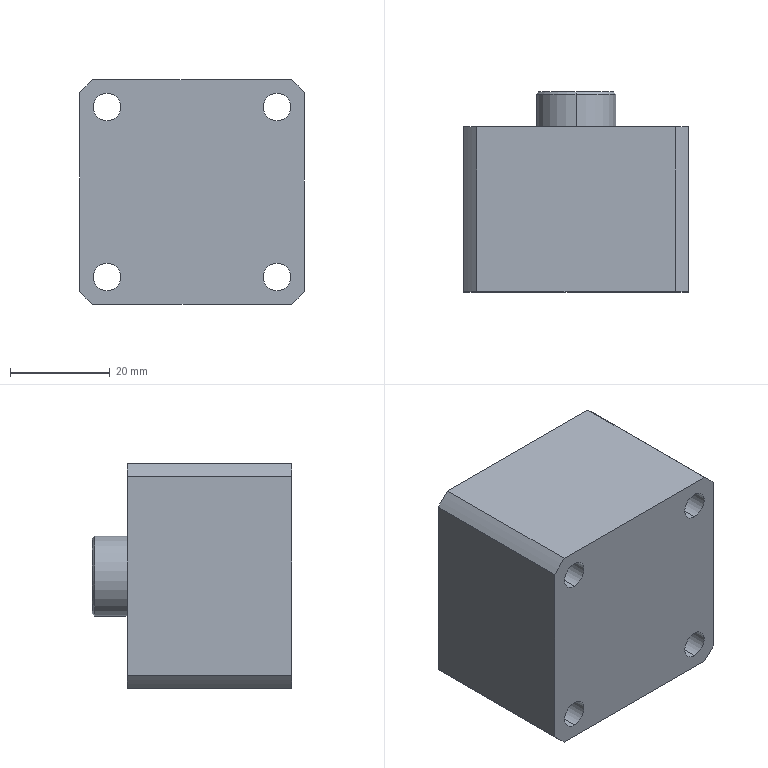Part | STEP file | CDQ2B32-10-A73 | 1 solid | 29 faces | box 44.99 x 40 x 44.982 mm | volume 63998 mm3 | cylinder 16 | plane 7 | cone 6 | commonest cylinder face diameters 5.5 x8 60 x4 6.8 x2 16 x2